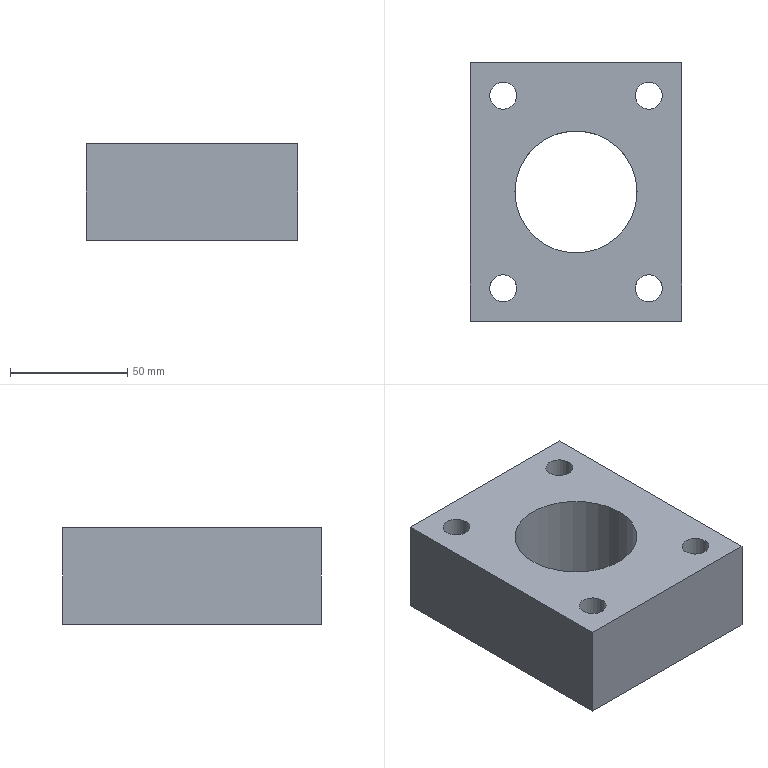Part | NX | features solid 2 | 1 solid | 19 faces | box 90 x 110 x 41 mm | volume 293962 mm3 | plane 10 | cylinder 9 | commonest cylinder face diameters 11.5 x4 18 x4 52 x1
STEP:
#1=CARTESIAN_POINT('',(1165.,-284.,60.));
#2=VERTEX_POINT('',#1);
#3=CARTESIAN_POINT('',(1156.,-284.,60.));
#4=DIRECTION('',(0.,0.,1.));
#5=DIRECTION('',(1.,0.,0.));
#6=AXIS2_PLACEMENT_3D('',#3,#4,#5);
#7=CIRCLE('',#6,9.);
#8=EDGE_CURVE('',#2,#2,#7,.T.);
#9=ORIENTED_EDGE('',*,*,#8,.T.);
#10=EDGE_LOOP('',(#9));
#11=FACE_BOUND('',#10,.T.);
#12=CARTESIAN_POINT('',(1103.,-366.,60.));
#13=VERTEX_POINT('',#12);
#14=CARTESIAN_POINT('',(1094.,-366.,60.));
#15=DIRECTION('',(0.,0.,1.));
#16=DIRECTION('',(1.,0.,0.));
#17=AXIS2_PLACEMENT_3D('',#14,#15,#16);
#18=CIRCLE('',#17,9.);
#19=EDGE_CURVE('',#13,#13,#18,.T.);
#20=ORIENTED_EDGE('',*,*,#19,.T.);
#21=EDGE_LOOP('',(#20));
#22=FACE_BOUND('',#21,.T.);
#23=CARTESIAN_POINT('',(1170.,-380.,60.));
#24=VERTEX_POINT('',#23);
#25=CARTESIAN_POINT('',(1170.,-270.,60.));
#26=VERTEX_POINT('',#25);
#27=CARTESIAN_POINT('',(1170.,-325.,60.));
#28=DIRECTION('',(0.,1.,0.));
#29=VECTOR('',#28,1000.);
#30=LINE('',#27,#29);
#31=EDGE_CURVE('',#24,#26,#30,.T.);
#32=ORIENTED_EDGE('',*,*,#31,.F.);
#33=CARTESIAN_POINT('',(1080.,-380.,60.));
#34=VERTEX_POINT('',#33);
#35=CARTESIAN_POINT('',(1125.,-380.,60.));
#36=DIRECTION('',(1.,0.,0.));
#37=VECTOR('',#36,1000.);
#38=LINE('',#35,#37);
#39=EDGE_CURVE('',#34,#24,#38,.T.);
#40=ORIENTED_EDGE('',*,*,#39,.F.);
#41=CARTESIAN_POINT('',(1080.,-270.,60.));
#42=VERTEX_POINT('',#41);
#43=CARTESIAN_POINT('',(1080.,-325.,60.));
#44=DIRECTION('',(0.,-1.,0.));
#45=VECTOR('',#44,1000.);
#46=LINE('',#43,#45);
#47=EDGE_CURVE('',#42,#34,#46,.T.);
#48=ORIENTED_EDGE('',*,*,#47,.F.);
#49=CARTESIAN_POINT('',(1125.,-270.,60.));
#50=DIRECTION('',(-1.,0.,0.));
#51=VECTOR('',#50,1000.);
#52=LINE('',#49,#51);
#53=EDGE_CURVE('',#26,#42,#52,.T.);
#54=ORIENTED_EDGE('',*,*,#53,.F.);
#55=EDGE_LOOP('',(#32,#40,#48,#54));
#56=FACE_BOUND('',#55,.T.);
#57=CARTESIAN_POINT('',(1151.,-325.,60.));
#58=VERTEX_POINT('',#57);
#59=CARTESIAN_POINT('',(1125.,-325.,60.));
#60=DIRECTION('',(0.,0.,1.));
#61=DIRECTION('',(1.,0.,0.));
#62=AXIS2_PLACEMENT_3D('',#59,#60,#61);
#63=CIRCLE('',#62,26.);
#64=EDGE_CURVE('',#58,#58,#63,.T.);
#65=ORIENTED_EDGE('',*,*,#64,.T.);
#66=EDGE_LOOP('',(#65));
#67=FACE_BOUND('',#66,.T.);
#68=CARTESIAN_POINT('',(1165.,-366.,60.));
#69=VERTEX_POINT('',#68);
#70=CARTESIAN_POINT('',(1156.,-366.,60.));
#71=DIRECTION('',(0.,0.,1.));
#72=DIRECTION('',(1.,0.,0.));
#73=AXIS2_PLACEMENT_3D('',#70,#71,#72);
#74=CIRCLE('',#73,9.);
#75=EDGE_CURVE('',#69,#69,#74,.T.);
#76=ORIENTED_EDGE('',*,*,#75,.T.);
#77=EDGE_LOOP('',(#76));
#78=FACE_BOUND('',#77,.T.);
#79=CARTESIAN_POINT('',(1103.,-284.,60.));
#80=VERTEX_POINT('',#79);
#81=CARTESIAN_POINT('',(1094.,-284.,60.));
#82=DIRECTION('',(0.,0.,1.));
#83=DIRECTION('',(1.,0.,0.));
#84=AXIS2_PLACEMENT_3D('',#81,#82,#83);
#85=CIRCLE('',#84,9.);
#86=EDGE_CURVE('',#80,#80,#85,.T.);
#87=ORIENTED_EDGE('',*,*,#86,.T.);
#88=EDGE_LOOP('',(#87));
#89=FACE_BOUND('',#88,.T.);
#90=CARTESIAN_POINT('',(2312.5,0.,60.));
#91=DIRECTION('',(0.,0.,1.));
#92=DIRECTION('',(-1.,0.,0.));
#93=AXIS2_PLACEMENT_3D('',#90,#91,#92);
#94=PLANE('',#93);
#95=ADVANCED_FACE('',(#11,#22,#56,#67,#78,#89),#94,.F.);
#96=CARTESIAN_POINT('',(1099.75,-284.,101.));
#97=VERTEX_POINT('',#96);
#98=CARTESIAN_POINT('',(1094.,-284.,101.));
#99=DIRECTION('',(0.,0.,1.));
#100=DIRECTION('',(1.,0.,0.));
#101=AXIS2_PLACEMENT_3D('',#98,#99,#100);
#102=CIRCLE('',#101,5.75);
#103=EDGE_CURVE('',#97,#97,#102,.T.);
#104=ORIENTED_EDGE('',*,*,#103,.F.);
#105=EDGE_LOOP('',(#104));
#106=FACE_BOUND('',#105,.T.);
#107=CARTESIAN_POINT('',(1161.75,-284.,101.));
#108=VERTEX_POINT('',#107);
#109=CARTESIAN_POINT('',(1156.,-284.,101.));
#110=DIRECTION('',(0.,0.,1.));
#111=DIRECTION('',(1.,0.,0.));
#112=AXIS2_PLACEMENT_3D('',#109,#110,#111);
#113=CIRCLE('',#112,5.75);
#114=EDGE_CURVE('',#108,#108,#113,.T.);
#115=ORIENTED_EDGE('',*,*,#114,.F.);
#116=EDGE_LOOP('',(#115));
#117=FACE_BOUND('',#116,.T.);
#118=CARTESIAN_POINT('',(1161.75,-366.,101.));
#119=VERTEX_POINT('',#118);
#120=CARTESIAN_POINT('',(1156.,-366.,101.));
#121=DIRECTION('',(0.,0.,1.));
#122=DIRECTION('',(1.,0.,0.));
#123=AXIS2_PLACEMENT_3D('',#120,#121,#122);
#124=CIRCLE('',#123,5.75);
#125=EDGE_CURVE('',#119,#119,#124,.T.);
#126=ORIENTED_EDGE('',*,*,#125,.F.);
#127=EDGE_LOOP('',(#126));
#128=FACE_BOUND('',#127,.T.);
#129=CARTESIAN_POINT('',(1099.75,-366.,101.));
#130=VERTEX_POINT('',#129);
#131=CARTESIAN_POINT('',(1094.,-366.,101.));
#132=DIRECTION('',(0.,0.,1.));
#133=DIRECTION('',(1.,0.,0.));
#134=AXIS2_PLACEMENT_3D('',#131,#132,#133);
#135=CIRCLE('',#134,5.75);
#136=EDGE_CURVE('',#130,#130,#135,.T.);
#137=ORIENTED_EDGE('',*,*,#136,.F.);
#138=EDGE_LOOP('',(#137));
#139=FACE_BOUND('',#138,.T.);
#140=CARTESIAN_POINT('',(1170.,-380.,101.));
#141=VERTEX_POINT('',#140);
#142=CARTESIAN_POINT('',(1080.,-380.,101.));
#143=VERTEX_POINT('',#142);
#144=CARTESIAN_POINT('',(1125.,-380.,101.));
#145=DIRECTION('',(-1.,0.,0.));
#146=VECTOR('',#145,1000.);
#147=LINE('',#144,#146);
#148=EDGE_CURVE('',#141,#143,#147,.T.);
#149=ORIENTED_EDGE('',*,*,#148,.F.);
#150=CARTESIAN_POINT('',(1170.,-270.,101.));
#151=VERTEX_POINT('',#150);
#152=CARTESIAN_POINT('',(1170.,-325.,101.));
#153=DIRECTION('',(0.,-1.,0.));
#154=VECTOR('',#153,1000.);
#155=LINE('',#152,#154);
#156=EDGE_CURVE('',#151,#141,#155,.T.);
#157=ORIENTED_EDGE('',*,*,#156,.F.);
#158=CARTESIAN_POINT('',(1080.,-270.,101.));
#159=VERTEX_POINT('',#158);
#160=CARTESIAN_POINT('',(1125.,-270.,101.));
#161=DIRECTION('',(1.,0.,0.));
#162=VECTOR('',#161,1000.);
#163=LINE('',#160,#162);
#164=EDGE_CURVE('',#159,#151,#163,.T.);
#165=ORIENTED_EDGE('',*,*,#164,.F.);
#166=CARTESIAN_POINT('',(1080.,-325.,101.));
#167=DIRECTION('',(0.,1.,0.));
#168=VECTOR('',#167,1000.);
#169=LINE('',#166,#168);
#170=EDGE_CURVE('',#143,#159,#169,.T.);
#171=ORIENTED_EDGE('',*,*,#170,.F.);
#172=EDGE_LOOP('',(#149,#157,#165,#171));
#173=FACE_BOUND('',#172,.T.);
#174=CARTESIAN_POINT('',(1151.,-325.,101.));
#175=VERTEX_POINT('',#174);
#176=CARTESIAN_POINT('',(1125.,-325.,101.));
#177=DIRECTION('',(0.,0.,-1.));
#178=DIRECTION('',(1.,0.,0.));
#179=AXIS2_PLACEMENT_3D('',#176,#177,#178);
#180=CIRCLE('',#179,26.);
#181=EDGE_CURVE('',#175,#175,#180,.T.);
#182=ORIENTED_EDGE('',*,*,#181,.T.);
#183=EDGE_LOOP('',(#182));
#184=FACE_BOUND('',#183,.T.);
#185=CARTESIAN_POINT('',(282.5,193.,101.));
#186=DIRECTION('',(0.,0.,1.));
#187=DIRECTION('',(-1.,0.,0.));
#188=AXIS2_PLACEMENT_3D('',#185,#186,#187);
#189=PLANE('',#188);
#190=ADVANCED_FACE('',(#106,#117,#128,#139,#173,#184),#189,.T.);
#191=CARTESIAN_POINT('',(1170.,-380.,-25.));
#192=DIRECTION('',(0.,0.,1.));
#193=VECTOR('',#192,1000.);
#194=LINE('',#191,#193);
#195=EDGE_CURVE('',#24,#141,#194,.T.);
#196=ORIENTED_EDGE('',*,*,#195,.T.);
#197=ORIENTED_EDGE('',*,*,#148,.T.);
#198=CARTESIAN_POINT('',(1080.,-380.,-25.));
#199=DIRECTION('',(0.,0.,1.));
#200=VECTOR('',#199,1000.);
#201=LINE('',#198,#200);
#202=EDGE_CURVE('',#34,#143,#201,.T.);
#203=ORIENTED_EDGE('',*,*,#202,.F.);
#204=ORIENTED_EDGE('',*,*,#39,.T.);
#205=EDGE_LOOP('',(#196,#197,#203,#204));
#206=FACE_BOUND('',#205,.T.);
#207=CARTESIAN_POINT('',(1125.,-380.,-25.));
#208=DIRECTION('',(0.,-1.,0.));
#209=DIRECTION('',(0.,0.,1.));
#210=AXIS2_PLACEMENT_3D('',#207,#208,#209);
#211=PLANE('',#210);
#212=ADVANCED_FACE('',(#206),#211,.T.);
#213=ORIENTED_EDGE('',*,*,#202,.T.);
#214=ORIENTED_EDGE('',*,*,#170,.T.);
#215=CARTESIAN_POINT('',(1080.,-270.,-25.));
#216=DIRECTION('',(0.,0.,1.));
#217=VECTOR('',#216,1000.);
#218=LINE('',#215,#217);
#219=EDGE_CURVE('',#42,#159,#218,.T.);
#220=ORIENTED_EDGE('',*,*,#219,.F.);
#221=ORIENTED_EDGE('',*,*,#47,.T.);
#222=EDGE_LOOP('',(#213,#214,#220,#221));
#223=FACE_BOUND('',#222,.T.);
#224=CARTESIAN_POINT('',(1080.,-325.,-25.));
#225=DIRECTION('',(-1.,0.,0.));
#226=DIRECTION('',(0.,0.,-1.));
#227=AXIS2_PLACEMENT_3D('',#224,#225,#226);
#228=PLANE('',#227);
#229=ADVANCED_FACE('',(#223),#228,.T.);
#230=ORIENTED_EDGE('',*,*,#219,.T.);
#231=ORIENTED_EDGE('',*,*,#164,.T.);
#232=CARTESIAN_POINT('',(1170.,-270.,-25.));
#233=DIRECTION('',(0.,0.,1.));
#234=VECTOR('',#233,1000.);
#235=LINE('',#232,#234);
#236=EDGE_CURVE('',#26,#151,#235,.T.);
#237=ORIENTED_EDGE('',*,*,#236,.F.);
#238=ORIENTED_EDGE('',*,*,#53,.T.);
#239=EDGE_LOOP('',(#230,#231,#237,#238));
#240=FACE_BOUND('',#239,.T.);
#241=CARTESIAN_POINT('',(1125.,-270.,-25.));
#242=DIRECTION('',(0.,1.,0.));
#243=DIRECTION('',(0.,0.,-1.));
#244=AXIS2_PLACEMENT_3D('',#241,#242,#243);
#245=PLANE('',#244);
#246=ADVANCED_FACE('',(#240),#245,.T.);
#247=ORIENTED_EDGE('',*,*,#31,.T.);
#248=ORIENTED_EDGE('',*,*,#236,.T.);
#249=ORIENTED_EDGE('',*,*,#156,.T.);
#250=ORIENTED_EDGE('',*,*,#195,.F.);
#251=EDGE_LOOP('',(#247,#248,#249,#250));
#252=FACE_BOUND('',#251,.T.);
#253=CARTESIAN_POINT('',(1170.,-325.,-25.));
#254=DIRECTION('',(1.,0.,0.));
#255=DIRECTION('',(0.,0.,1.));
#256=AXIS2_PLACEMENT_3D('',#253,#254,#255);
#257=PLANE('',#256);
#258=ADVANCED_FACE('',(#252),#257,.T.);
#259=ORIENTED_EDGE('',*,*,#181,.F.);
#260=EDGE_LOOP('',(#259));
#261=FACE_BOUND('',#260,.T.);
#262=ORIENTED_EDGE('',*,*,#64,.F.);
#263=EDGE_LOOP('',(#262));
#264=FACE_BOUND('',#263,.T.);
#265=CARTESIAN_POINT('',(1125.,-325.,-181.));
#266=DIRECTION('',(0.,0.,1.));
#267=DIRECTION('',(-1.,0.,0.));
#268=AXIS2_PLACEMENT_3D('',#265,#266,#267);
#269=CYLINDRICAL_SURFACE('',#268,26.);
#270=ADVANCED_FACE('',(#261,#264),#269,.F.);
#271=ORIENTED_EDGE('',*,*,#136,.T.);
#272=EDGE_LOOP('',(#271));
#273=FACE_BOUND('',#272,.T.);
#274=CARTESIAN_POINT('',(1099.75,-366.,73.));
#275=VERTEX_POINT('',#274);
#276=CARTESIAN_POINT('',(1094.,-366.,73.));
#277=DIRECTION('',(0.,0.,1.));
#278=DIRECTION('',(1.,0.,0.));
#279=AXIS2_PLACEMENT_3D('',#276,#277,#278);
#280=CIRCLE('',#279,5.75);
#281=EDGE_CURVE('',#275,#275,#280,.T.);
#282=ORIENTED_EDGE('',*,*,#281,.F.);
#283=EDGE_LOOP('',(#282));
#284=FACE_BOUND('',#283,.T.);
#285=CARTESIAN_POINT('',(1094.,-366.,55.));
#286=DIRECTION('',(0.,0.,1.));
#287=DIRECTION('',(-1.,0.,0.));
#288=AXIS2_PLACEMENT_3D('',#285,#286,#287);
#289=CYLINDRICAL_SURFACE('',#288,5.75);
#290=ADVANCED_FACE('',(#273,#284),#289,.F.);
#291=ORIENTED_EDGE('',*,*,#281,.T.);
#292=EDGE_LOOP('',(#291));
#293=FACE_BOUND('',#292,.T.);
#294=CARTESIAN_POINT('',(1103.,-366.,73.));
#295=VERTEX_POINT('',#294);
#296=CARTESIAN_POINT('',(1094.,-366.,73.));
#297=DIRECTION('',(0.,0.,1.));
#298=DIRECTION('',(1.,0.,0.));
#299=AXIS2_PLACEMENT_3D('',#296,#297,#298);
#300=CIRCLE('',#299,9.);
#301=EDGE_CURVE('',#295,#295,#300,.T.);
#302=ORIENTED_EDGE('',*,*,#301,.F.);
#303=EDGE_LOOP('',(#302));
#304=FACE_BOUND('',#303,.T.);
#305=CARTESIAN_POINT('',(1094.,-366.,73.));
#306=DIRECTION('',(0.,0.,1.));
#307=DIRECTION('',(-1.,0.,0.));
#308=AXIS2_PLACEMENT_3D('',#305,#306,#307);
#309=PLANE('',#308);
#310=ADVANCED_FACE('',(#293,#304),#309,.F.);
#311=ORIENTED_EDGE('',*,*,#301,.T.);
#312=EDGE_LOOP('',(#311));
#313=FACE_BOUND('',#312,.T.);
#314=ORIENTED_EDGE('',*,*,#19,.F.);
#315=EDGE_LOOP('',(#314));
#316=FACE_BOUND('',#315,.T.);
#317=CARTESIAN_POINT('',(1094.,-366.,60.));
#318=DIRECTION('',(0.,0.,1.));
#319=DIRECTION('',(-1.,0.,0.));
#320=AXIS2_PLACEMENT_3D('',#317,#318,#319);
#321=CYLINDRICAL_SURFACE('',#320,9.);
#322=ADVANCED_FACE('',(#313,#316),#321,.F.);
#323=ORIENTED_EDGE('',*,*,#125,.T.);
#324=EDGE_LOOP('',(#323));
#325=FACE_BOUND('',#324,.T.);
#326=CARTESIAN_POINT('',(1161.75,-366.,73.));
#327=VERTEX_POINT('',#326);
#328=CARTESIAN_POINT('',(1156.,-366.,73.));
#329=DIRECTION('',(0.,0.,1.));
#330=DIRECTION('',(1.,0.,0.));
#331=AXIS2_PLACEMENT_3D('',#328,#329,#330);
#332=CIRCLE('',#331,5.75);
#333=EDGE_CURVE('',#327,#327,#332,.T.);
#334=ORIENTED_EDGE('',*,*,#333,.F.);
#335=EDGE_LOOP('',(#334));
#336=FACE_BOUND('',#335,.T.);
#337=CARTESIAN_POINT('',(1156.,-366.,55.));
#338=DIRECTION('',(0.,0.,1.));
#339=DIRECTION('',(-1.,0.,0.));
#340=AXIS2_PLACEMENT_3D('',#337,#338,#339);
#341=CYLINDRICAL_SURFACE('',#340,5.75);
#342=ADVANCED_FACE('',(#325,#336),#341,.F.);
#343=ORIENTED_EDGE('',*,*,#333,.T.);
#344=EDGE_LOOP('',(#343));
#345=FACE_BOUND('',#344,.T.);
#346=CARTESIAN_POINT('',(1165.,-366.,73.));
#347=VERTEX_POINT('',#346);
#348=CARTESIAN_POINT('',(1156.,-366.,73.));
#349=DIRECTION('',(0.,0.,1.));
#350=DIRECTION('',(1.,0.,0.));
#351=AXIS2_PLACEMENT_3D('',#348,#349,#350);
#352=CIRCLE('',#351,9.);
#353=EDGE_CURVE('',#347,#347,#352,.T.);
#354=ORIENTED_EDGE('',*,*,#353,.F.);
#355=EDGE_LOOP('',(#354));
#356=FACE_BOUND('',#355,.T.);
#357=CARTESIAN_POINT('',(1156.,-366.,73.));
#358=DIRECTION('',(0.,0.,1.));
#359=DIRECTION('',(-1.,0.,0.));
#360=AXIS2_PLACEMENT_3D('',#357,#358,#359);
#361=PLANE('',#360);
#362=ADVANCED_FACE('',(#345,#356),#361,.F.);
#363=ORIENTED_EDGE('',*,*,#353,.T.);
#364=EDGE_LOOP('',(#363));
#365=FACE_BOUND('',#364,.T.);
#366=ORIENTED_EDGE('',*,*,#75,.F.);
#367=EDGE_LOOP('',(#366));
#368=FACE_BOUND('',#367,.T.);
#369=CARTESIAN_POINT('',(1156.,-366.,60.));
#370=DIRECTION('',(0.,0.,1.));
#371=DIRECTION('',(-1.,0.,0.));
#372=AXIS2_PLACEMENT_3D('',#369,#370,#371);
#373=CYLINDRICAL_SURFACE('',#372,9.);
#374=ADVANCED_FACE('',(#365,#368),#373,.F.);
#375=ORIENTED_EDGE('',*,*,#114,.T.);
#376=EDGE_LOOP('',(#375));
#377=FACE_BOUND('',#376,.T.);
#378=CARTESIAN_POINT('',(1161.75,-284.,73.));
#379=VERTEX_POINT('',#378);
#380=CARTESIAN_POINT('',(1156.,-284.,73.));
#381=DIRECTION('',(0.,0.,1.));
#382=DIRECTION('',(1.,0.,0.));
#383=AXIS2_PLACEMENT_3D('',#380,#381,#382);
#384=CIRCLE('',#383,5.75);
#385=EDGE_CURVE('',#379,#379,#384,.T.);
#386=ORIENTED_EDGE('',*,*,#385,.F.);
#387=EDGE_LOOP('',(#386));
#388=FACE_BOUND('',#387,.T.);
#389=CARTESIAN_POINT('',(1156.,-284.,55.));
#390=DIRECTION('',(0.,0.,1.));
#391=DIRECTION('',(-1.,0.,0.));
#392=AXIS2_PLACEMENT_3D('',#389,#390,#391);
#393=CYLINDRICAL_SURFACE('',#392,5.75);
#394=ADVANCED_FACE('',(#377,#388),#393,.F.);
#395=ORIENTED_EDGE('',*,*,#385,.T.);
#396=EDGE_LOOP('',(#395));
#397=FACE_BOUND('',#396,.T.);
#398=CARTESIAN_POINT('',(1165.,-284.,73.));
#399=VERTEX_POINT('',#398);
#400=CARTESIAN_POINT('',(1156.,-284.,73.));
#401=DIRECTION('',(0.,0.,1.));
#402=DIRECTION('',(1.,0.,0.));
#403=AXIS2_PLACEMENT_3D('',#400,#401,#402);
#404=CIRCLE('',#403,9.);
#405=EDGE_CURVE('',#399,#399,#404,.T.);
#406=ORIENTED_EDGE('',*,*,#405,.F.);
#407=EDGE_LOOP('',(#406));
#408=FACE_BOUND('',#407,.T.);
#409=CARTESIAN_POINT('',(1156.,-284.,73.));
#410=DIRECTION('',(0.,0.,1.));
#411=DIRECTION('',(-1.,0.,0.));
#412=AXIS2_PLACEMENT_3D('',#409,#410,#411);
#413=PLANE('',#412);
#414=ADVANCED_FACE('',(#397,#408),#413,.F.);
#415=ORIENTED_EDGE('',*,*,#405,.T.);
#416=EDGE_LOOP('',(#415));
#417=FACE_BOUND('',#416,.T.);
#418=ORIENTED_EDGE('',*,*,#8,.F.);
#419=EDGE_LOOP('',(#418));
#420=FACE_BOUND('',#419,.T.);
#421=CARTESIAN_POINT('',(1156.,-284.,60.));
#422=DIRECTION('',(0.,0.,1.));
#423=DIRECTION('',(-1.,0.,0.));
#424=AXIS2_PLACEMENT_3D('',#421,#422,#423);
#425=CYLINDRICAL_SURFACE('',#424,9.);
#426=ADVANCED_FACE('',(#417,#420),#425,.F.);
#427=ORIENTED_EDGE('',*,*,#103,.T.);
#428=EDGE_LOOP('',(#427));
#429=FACE_BOUND('',#428,.T.);
#430=CARTESIAN_POINT('',(1099.75,-284.,73.));
#431=VERTEX_POINT('',#430);
#432=CARTESIAN_POINT('',(1094.,-284.,73.));
#433=DIRECTION('',(0.,0.,1.));
#434=DIRECTION('',(1.,0.,0.));
#435=AXIS2_PLACEMENT_3D('',#432,#433,#434);
#436=CIRCLE('',#435,5.75);
#437=EDGE_CURVE('',#431,#431,#436,.T.);
#438=ORIENTED_EDGE('',*,*,#437,.F.);
#439=EDGE_LOOP('',(#438));
#440=FACE_BOUND('',#439,.T.);
#441=CARTESIAN_POINT('',(1094.,-284.,55.));
#442=DIRECTION('',(0.,0.,1.));
#443=DIRECTION('',(-1.,0.,0.));
#444=AXIS2_PLACEMENT_3D('',#441,#442,#443);
#445=CYLINDRICAL_SURFACE('',#444,5.75);
#446=ADVANCED_FACE('',(#429,#440),#445,.F.);
#447=ORIENTED_EDGE('',*,*,#437,.T.);
#448=EDGE_LOOP('',(#447));
#449=FACE_BOUND('',#448,.T.);
#450=CARTESIAN_POINT('',(1103.,-284.,73.));
#451=VERTEX_POINT('',#450);
#452=CARTESIAN_POINT('',(1094.,-284.,73.));
#453=DIRECTION('',(0.,0.,1.));
#454=DIRECTION('',(1.,0.,0.));
#455=AXIS2_PLACEMENT_3D('',#452,#453,#454);
#456=CIRCLE('',#455,9.);
#457=EDGE_CURVE('',#451,#451,#456,.T.);
#458=ORIENTED_EDGE('',*,*,#457,.F.);
#459=EDGE_LOOP('',(#458));
#460=FACE_BOUND('',#459,.T.);
#461=CARTESIAN_POINT('',(1094.,-284.,73.));
#462=DIRECTION('',(0.,0.,1.));
#463=DIRECTION('',(-1.,0.,0.));
#464=AXIS2_PLACEMENT_3D('',#461,#462,#463);
#465=PLANE('',#464);
#466=ADVANCED_FACE('',(#449,#460),#465,.F.);
#467=ORIENTED_EDGE('',*,*,#457,.T.);
#468=EDGE_LOOP('',(#467));
#469=FACE_BOUND('',#468,.T.);
#470=ORIENTED_EDGE('',*,*,#86,.F.);
#471=EDGE_LOOP('',(#470));
#472=FACE_BOUND('',#471,.T.);
#473=CARTESIAN_POINT('',(1094.,-284.,60.));
#474=DIRECTION('',(0.,0.,1.));
#475=DIRECTION('',(-1.,0.,0.));
#476=AXIS2_PLACEMENT_3D('',#473,#474,#475);
#477=CYLINDRICAL_SURFACE('',#476,9.);
#478=ADVANCED_FACE('',(#469,#472),#477,.F.);
#479=CLOSED_SHELL('',(#95,#190,#212,#229,#246,#258,#270,#290,#310,#322,#342,#362,#374,#394,#414,#426,#446,#466,#478));
#480=MANIFOLD_SOLID_BREP('',#479);
#481=(LENGTH_UNIT()NAMED_UNIT(*)SI_UNIT(.MILLI.,.METRE.));
#482=UNCERTAINTY_MEASURE_WITH_UNIT(LENGTH_MEASURE(0.00001),#481,'','');
#483=(NAMED_UNIT(*)PLANE_ANGLE_UNIT()SI_UNIT($,.RADIAN.));
#484=(NAMED_UNIT(*)SI_UNIT($,.STERADIAN.)SOLID_ANGLE_UNIT());
#485=(GEOMETRIC_REPRESENTATION_CONTEXT(3)GLOBAL_UNCERTAINTY_ASSIGNED_CONTEXT((#482))GLOBAL_UNIT_ASSIGNED_CONTEXT((#481,#483,#484))REPRESENTATION_CONTEXT('',''));
#486=ADVANCED_BREP_SHAPE_REPRESENTATION('',(#480),#485);